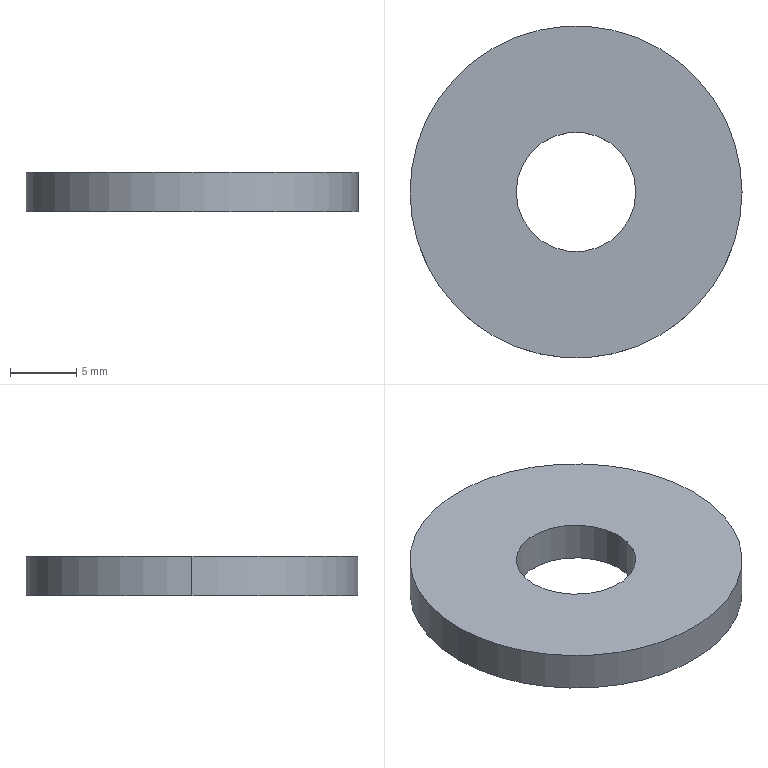Part | STEP file | Cuon T phu H01_15 | 1 solid | 6 faces | box 25 x 25 x 3 mm | volume 1282 mm3 | cylinder 4 | plane 2 | commonest cylinder face diameters 9 x2 25 x2
STEP:
#1=CARTESIAN_POINT('',(0.,0.,0.));
#2=DIRECTION('',(0.,0.,1.));
#3=DIRECTION('',(1.,0.,0.));
#4=AXIS2_PLACEMENT_3D('',#1,#2,#3);
#5=CARTESIAN_POINT('',(-4.5,0.,3.));
#6=VERTEX_POINT('',#5);
#7=CARTESIAN_POINT('',(-4.5,0.,0.));
#8=VERTEX_POINT('',#7);
#9=CARTESIAN_POINT('',(-4.5,0.,3.));
#10=DIRECTION('',(0.,0.,-1.));
#11=VECTOR('',#10,1.);
#12=LINE('',#9,#11);
#13=CARTESIAN_POINT('',(0.,0.,3.));
#14=DIRECTION('',(0.,0.,-1.));
#15=DIRECTION('',(-1.,0.,0.));
#16=AXIS2_PLACEMENT_3D('',#13,#14,#15);
#17=CYLINDRICAL_SURFACE('',#16,4.5);
#18=CARTESIAN_POINT('',(6.283,0.));
#19=DIRECTION('',(0.,1.));
#20=VECTOR('',#19,1.);
#21=LINE('',#18,#20);
#22=(GEOMETRIC_REPRESENTATION_CONTEXT(2)PARAMETRIC_REPRESENTATION_CONTEXT()REPRESENTATION_CONTEXT('',''));
#23=DEFINITIONAL_REPRESENTATION('',(#21),#22);
#24=PCURVE('',#17,#23);
#25=CARTESIAN_POINT('',(0.,0.,3.));
#26=DIRECTION('',(0.,0.,-1.));
#27=DIRECTION('',(-1.,0.,0.));
#28=AXIS2_PLACEMENT_3D('',#25,#26,#27);
#29=CYLINDRICAL_SURFACE('',#28,4.5);
#30=CARTESIAN_POINT('',(0.,0.));
#31=DIRECTION('',(0.,1.));
#32=VECTOR('',#31,1.);
#33=LINE('',#30,#32);
#34=(GEOMETRIC_REPRESENTATION_CONTEXT(2)PARAMETRIC_REPRESENTATION_CONTEXT()REPRESENTATION_CONTEXT('',''));
#35=DEFINITIONAL_REPRESENTATION('',(#33),#34);
#36=PCURVE('',#29,#35);
#37=SURFACE_CURVE('',#12,(#24,#36),.PCURVE_S1.);
#38=EDGE_CURVE('',#6,#8,#37,.T.);
#39=ORIENTED_EDGE('',*,*,#38,.T.);
#40=CARTESIAN_POINT('',(4.5,0.,0.));
#41=VERTEX_POINT('',#40);
#42=CARTESIAN_POINT('',(0.,0.,0.));
#43=DIRECTION('',(0.,0.,1.));
#44=DIRECTION('',(1.,0.,0.));
#45=AXIS2_PLACEMENT_3D('',#42,#43,#44);
#46=CIRCLE('',#45,4.5);
#47=CARTESIAN_POINT('',(9.425,3.));
#48=DIRECTION('',(-1.,0.));
#49=VECTOR('',#48,1.);
#50=LINE('',#47,#49);
#51=(GEOMETRIC_REPRESENTATION_CONTEXT(2)PARAMETRIC_REPRESENTATION_CONTEXT()REPRESENTATION_CONTEXT('',''));
#52=DEFINITIONAL_REPRESENTATION('',(#50),#51);
#53=PCURVE('',#17,#52);
#54=CARTESIAN_POINT('',(0.,0.,0.));
#55=DIRECTION('',(0.,0.,1.));
#56=DIRECTION('',(1.,0.,0.));
#57=AXIS2_PLACEMENT_3D('',#54,#55,#56);
#58=PLANE('',#57);
#59=CARTESIAN_POINT('',(0.,0.));
#60=DIRECTION('',(1.,0.));
#61=AXIS2_PLACEMENT_2D('',#59,#60);
#62=CIRCLE('',#61,4.5);
#63=(GEOMETRIC_REPRESENTATION_CONTEXT(2)PARAMETRIC_REPRESENTATION_CONTEXT()REPRESENTATION_CONTEXT('',''));
#64=DEFINITIONAL_REPRESENTATION('',(#62),#63);
#65=PCURVE('',#58,#64);
#66=SURFACE_CURVE('',#46,(#53,#65),.PCURVE_S1.);
#67=EDGE_CURVE('',#8,#41,#66,.T.);
#68=ORIENTED_EDGE('',*,*,#67,.T.);
#69=CARTESIAN_POINT('',(4.5,0.,3.));
#70=VERTEX_POINT('',#69);
#71=CARTESIAN_POINT('',(4.5,0.,3.));
#72=DIRECTION('',(0.,0.,-1.));
#73=VECTOR('',#72,1.);
#74=LINE('',#71,#73);
#75=CARTESIAN_POINT('',(3.142,0.));
#76=DIRECTION('',(0.,1.));
#77=VECTOR('',#76,1.);
#78=LINE('',#75,#77);
#79=(GEOMETRIC_REPRESENTATION_CONTEXT(2)PARAMETRIC_REPRESENTATION_CONTEXT()REPRESENTATION_CONTEXT('',''));
#80=DEFINITIONAL_REPRESENTATION('',(#78),#79);
#81=PCURVE('',#17,#80);
#82=CARTESIAN_POINT('',(3.142,0.));
#83=DIRECTION('',(0.,1.));
#84=VECTOR('',#83,1.);
#85=LINE('',#82,#84);
#86=(GEOMETRIC_REPRESENTATION_CONTEXT(2)PARAMETRIC_REPRESENTATION_CONTEXT()REPRESENTATION_CONTEXT('',''));
#87=DEFINITIONAL_REPRESENTATION('',(#85),#86);
#88=PCURVE('',#29,#87);
#89=SURFACE_CURVE('',#74,(#81,#88),.PCURVE_S1.);
#90=EDGE_CURVE('',#70,#41,#89,.T.);
#91=ORIENTED_EDGE('',*,*,#90,.F.);
#92=CARTESIAN_POINT('',(0.,0.,3.));
#93=DIRECTION('',(0.,0.,1.));
#94=DIRECTION('',(1.,0.,0.));
#95=AXIS2_PLACEMENT_3D('',#92,#93,#94);
#96=CIRCLE('',#95,4.5);
#97=CARTESIAN_POINT('',(9.425,0.));
#98=DIRECTION('',(-1.,0.));
#99=VECTOR('',#98,1.);
#100=LINE('',#97,#99);
#101=(GEOMETRIC_REPRESENTATION_CONTEXT(2)PARAMETRIC_REPRESENTATION_CONTEXT()REPRESENTATION_CONTEXT('',''));
#102=DEFINITIONAL_REPRESENTATION('',(#100),#101);
#103=PCURVE('',#17,#102);
#104=CARTESIAN_POINT('',(0.,0.,3.));
#105=DIRECTION('',(0.,0.,1.));
#106=DIRECTION('',(1.,0.,0.));
#107=AXIS2_PLACEMENT_3D('',#104,#105,#106);
#108=PLANE('',#107);
#109=CARTESIAN_POINT('',(0.,0.));
#110=DIRECTION('',(1.,0.));
#111=AXIS2_PLACEMENT_2D('',#109,#110);
#112=CIRCLE('',#111,4.5);
#113=(GEOMETRIC_REPRESENTATION_CONTEXT(2)PARAMETRIC_REPRESENTATION_CONTEXT()REPRESENTATION_CONTEXT('',''));
#114=DEFINITIONAL_REPRESENTATION('',(#112),#113);
#115=PCURVE('',#108,#114);
#116=SURFACE_CURVE('',#96,(#103,#115),.PCURVE_S1.);
#117=EDGE_CURVE('',#6,#70,#116,.T.);
#118=ORIENTED_EDGE('',*,*,#117,.F.);
#119=EDGE_LOOP('',(#39,#68,#91,#118));
#120=FACE_BOUND('',#119,.F.);
#121=ADVANCED_FACE('',(#120),#17,.F.);
#122=CARTESIAN_POINT('',(12.5,0.,3.));
#123=VERTEX_POINT('',#122);
#124=CARTESIAN_POINT('',(-12.5,0.,3.));
#125=VERTEX_POINT('',#124);
#126=CARTESIAN_POINT('',(0.,0.,3.));
#127=DIRECTION('',(0.,0.,1.));
#128=DIRECTION('',(1.,0.,0.));
#129=AXIS2_PLACEMENT_3D('',#126,#127,#128);
#130=CIRCLE('',#129,12.5);
#131=CARTESIAN_POINT('',(0.,0.,3.));
#132=DIRECTION('',(0.,0.,-1.));
#133=DIRECTION('',(-1.,0.,0.));
#134=AXIS2_PLACEMENT_3D('',#131,#132,#133);
#135=CYLINDRICAL_SURFACE('',#134,12.5);
#136=CARTESIAN_POINT('',(3.142,0.));
#137=DIRECTION('',(-1.,0.));
#138=VECTOR('',#137,1.);
#139=LINE('',#136,#138);
#140=(GEOMETRIC_REPRESENTATION_CONTEXT(2)PARAMETRIC_REPRESENTATION_CONTEXT()REPRESENTATION_CONTEXT('',''));
#141=DEFINITIONAL_REPRESENTATION('',(#139),#140);
#142=PCURVE('',#135,#141);
#143=CARTESIAN_POINT('',(0.,0.));
#144=DIRECTION('',(1.,0.));
#145=AXIS2_PLACEMENT_2D('',#143,#144);
#146=CIRCLE('',#145,12.5);
#147=(GEOMETRIC_REPRESENTATION_CONTEXT(2)PARAMETRIC_REPRESENTATION_CONTEXT()REPRESENTATION_CONTEXT('',''));
#148=DEFINITIONAL_REPRESENTATION('',(#146),#147);
#149=PCURVE('',#108,#148);
#150=SURFACE_CURVE('',#130,(#142,#149),.PCURVE_S1.);
#151=EDGE_CURVE('',#123,#125,#150,.T.);
#152=ORIENTED_EDGE('',*,*,#151,.F.);
#153=CARTESIAN_POINT('',(12.5,0.,0.));
#154=VERTEX_POINT('',#153);
#155=CARTESIAN_POINT('',(12.5,0.,3.));
#156=DIRECTION('',(0.,0.,-1.));
#157=VECTOR('',#156,1.);
#158=LINE('',#155,#157);
#159=CARTESIAN_POINT('',(3.142,0.));
#160=DIRECTION('',(0.,1.));
#161=VECTOR('',#160,1.);
#162=LINE('',#159,#161);
#163=(GEOMETRIC_REPRESENTATION_CONTEXT(2)PARAMETRIC_REPRESENTATION_CONTEXT()REPRESENTATION_CONTEXT('',''));
#164=DEFINITIONAL_REPRESENTATION('',(#162),#163);
#165=PCURVE('',#135,#164);
#166=CARTESIAN_POINT('',(0.,0.,3.));
#167=DIRECTION('',(0.,0.,-1.));
#168=DIRECTION('',(-1.,0.,0.));
#169=AXIS2_PLACEMENT_3D('',#166,#167,#168);
#170=CYLINDRICAL_SURFACE('',#169,12.5);
#171=CARTESIAN_POINT('',(3.142,0.));
#172=DIRECTION('',(0.,1.));
#173=VECTOR('',#172,1.);
#174=LINE('',#171,#173);
#175=(GEOMETRIC_REPRESENTATION_CONTEXT(2)PARAMETRIC_REPRESENTATION_CONTEXT()REPRESENTATION_CONTEXT('',''));
#176=DEFINITIONAL_REPRESENTATION('',(#174),#175);
#177=PCURVE('',#170,#176);
#178=SURFACE_CURVE('',#158,(#165,#177),.PCURVE_S1.);
#179=EDGE_CURVE('',#123,#154,#178,.T.);
#180=ORIENTED_EDGE('',*,*,#179,.T.);
#181=CARTESIAN_POINT('',(-12.5,0.,0.));
#182=VERTEX_POINT('',#181);
#183=CARTESIAN_POINT('',(0.,0.,0.));
#184=DIRECTION('',(0.,0.,1.));
#185=DIRECTION('',(1.,0.,0.));
#186=AXIS2_PLACEMENT_3D('',#183,#184,#185);
#187=CIRCLE('',#186,12.5);
#188=CARTESIAN_POINT('',(3.142,3.));
#189=DIRECTION('',(-1.,0.));
#190=VECTOR('',#189,1.);
#191=LINE('',#188,#190);
#192=(GEOMETRIC_REPRESENTATION_CONTEXT(2)PARAMETRIC_REPRESENTATION_CONTEXT()REPRESENTATION_CONTEXT('',''));
#193=DEFINITIONAL_REPRESENTATION('',(#191),#192);
#194=PCURVE('',#135,#193);
#195=CARTESIAN_POINT('',(0.,0.));
#196=DIRECTION('',(1.,0.));
#197=AXIS2_PLACEMENT_2D('',#195,#196);
#198=CIRCLE('',#197,12.5);
#199=(GEOMETRIC_REPRESENTATION_CONTEXT(2)PARAMETRIC_REPRESENTATION_CONTEXT()REPRESENTATION_CONTEXT('',''));
#200=DEFINITIONAL_REPRESENTATION('',(#198),#199);
#201=PCURVE('',#58,#200);
#202=SURFACE_CURVE('',#187,(#194,#201),.PCURVE_S1.);
#203=EDGE_CURVE('',#154,#182,#202,.T.);
#204=ORIENTED_EDGE('',*,*,#203,.T.);
#205=CARTESIAN_POINT('',(-12.5,0.,3.));
#206=DIRECTION('',(0.,0.,-1.));
#207=VECTOR('',#206,1.);
#208=LINE('',#205,#207);
#209=CARTESIAN_POINT('',(0.,0.));
#210=DIRECTION('',(0.,1.));
#211=VECTOR('',#210,1.);
#212=LINE('',#209,#211);
#213=(GEOMETRIC_REPRESENTATION_CONTEXT(2)PARAMETRIC_REPRESENTATION_CONTEXT()REPRESENTATION_CONTEXT('',''));
#214=DEFINITIONAL_REPRESENTATION('',(#212),#213);
#215=PCURVE('',#135,#214);
#216=CARTESIAN_POINT('',(6.283,0.));
#217=DIRECTION('',(0.,1.));
#218=VECTOR('',#217,1.);
#219=LINE('',#216,#218);
#220=(GEOMETRIC_REPRESENTATION_CONTEXT(2)PARAMETRIC_REPRESENTATION_CONTEXT()REPRESENTATION_CONTEXT('',''));
#221=DEFINITIONAL_REPRESENTATION('',(#219),#220);
#222=PCURVE('',#170,#221);
#223=SURFACE_CURVE('',#208,(#215,#222),.PCURVE_S1.);
#224=EDGE_CURVE('',#125,#182,#223,.T.);
#225=ORIENTED_EDGE('',*,*,#224,.F.);
#226=EDGE_LOOP('',(#152,#180,#204,#225));
#227=FACE_BOUND('',#226,.T.);
#228=ADVANCED_FACE('',(#227),#135,.T.);
#229=CARTESIAN_POINT('',(0.,0.,3.));
#230=DIRECTION('',(0.,0.,1.));
#231=DIRECTION('',(1.,0.,0.));
#232=AXIS2_PLACEMENT_3D('',#229,#230,#231);
#233=CIRCLE('',#232,12.5);
#234=CARTESIAN_POINT('',(0.,0.));
#235=DIRECTION('',(1.,0.));
#236=AXIS2_PLACEMENT_2D('',#234,#235);
#237=CIRCLE('',#236,12.5);
#238=(GEOMETRIC_REPRESENTATION_CONTEXT(2)PARAMETRIC_REPRESENTATION_CONTEXT()REPRESENTATION_CONTEXT('',''));
#239=DEFINITIONAL_REPRESENTATION('',(#237),#238);
#240=PCURVE('',#108,#239);
#241=CARTESIAN_POINT('',(9.425,0.));
#242=DIRECTION('',(-1.,0.));
#243=VECTOR('',#242,1.);
#244=LINE('',#241,#243);
#245=(GEOMETRIC_REPRESENTATION_CONTEXT(2)PARAMETRIC_REPRESENTATION_CONTEXT()REPRESENTATION_CONTEXT('',''));
#246=DEFINITIONAL_REPRESENTATION('',(#244),#245);
#247=PCURVE('',#170,#246);
#248=SURFACE_CURVE('',#233,(#240,#247),.PCURVE_S1.);
#249=EDGE_CURVE('',#125,#123,#248,.T.);
#250=ORIENTED_EDGE('',*,*,#249,.T.);
#251=ORIENTED_EDGE('',*,*,#151,.T.);
#252=EDGE_LOOP('',(#250,#251));
#253=FACE_BOUND('',#252,.T.);
#254=ORIENTED_EDGE('',*,*,#117,.F.);
#255=CARTESIAN_POINT('',(0.,0.,3.));
#256=DIRECTION('',(0.,0.,1.));
#257=DIRECTION('',(1.,0.,0.));
#258=AXIS2_PLACEMENT_3D('',#255,#256,#257);
#259=CIRCLE('',#258,4.5);
#260=CARTESIAN_POINT('',(0.,0.));
#261=DIRECTION('',(1.,0.));
#262=AXIS2_PLACEMENT_2D('',#260,#261);
#263=CIRCLE('',#262,4.5);
#264=(GEOMETRIC_REPRESENTATION_CONTEXT(2)PARAMETRIC_REPRESENTATION_CONTEXT()REPRESENTATION_CONTEXT('',''));
#265=DEFINITIONAL_REPRESENTATION('',(#263),#264);
#266=PCURVE('',#108,#265);
#267=CARTESIAN_POINT('',(3.142,0.));
#268=DIRECTION('',(-1.,0.));
#269=VECTOR('',#268,1.);
#270=LINE('',#267,#269);
#271=(GEOMETRIC_REPRESENTATION_CONTEXT(2)PARAMETRIC_REPRESENTATION_CONTEXT()REPRESENTATION_CONTEXT('',''));
#272=DEFINITIONAL_REPRESENTATION('',(#270),#271);
#273=PCURVE('',#29,#272);
#274=SURFACE_CURVE('',#259,(#266,#273),.PCURVE_S1.);
#275=EDGE_CURVE('',#70,#6,#274,.T.);
#276=ORIENTED_EDGE('',*,*,#275,.F.);
#277=EDGE_LOOP('',(#254,#276));
#278=FACE_BOUND('',#277,.T.);
#279=ADVANCED_FACE('',(#253,#278),#108,.T.);
#280=CARTESIAN_POINT('',(0.,0.,0.));
#281=DIRECTION('',(0.,0.,1.));
#282=DIRECTION('',(1.,0.,0.));
#283=AXIS2_PLACEMENT_3D('',#280,#281,#282);
#284=CIRCLE('',#283,12.5);
#285=CARTESIAN_POINT('',(0.,0.));
#286=DIRECTION('',(1.,0.));
#287=AXIS2_PLACEMENT_2D('',#285,#286);
#288=CIRCLE('',#287,12.5);
#289=(GEOMETRIC_REPRESENTATION_CONTEXT(2)PARAMETRIC_REPRESENTATION_CONTEXT()REPRESENTATION_CONTEXT('',''));
#290=DEFINITIONAL_REPRESENTATION('',(#288),#289);
#291=PCURVE('',#58,#290);
#292=CARTESIAN_POINT('',(9.425,3.));
#293=DIRECTION('',(-1.,0.));
#294=VECTOR('',#293,1.);
#295=LINE('',#292,#294);
#296=(GEOMETRIC_REPRESENTATION_CONTEXT(2)PARAMETRIC_REPRESENTATION_CONTEXT()REPRESENTATION_CONTEXT('',''));
#297=DEFINITIONAL_REPRESENTATION('',(#295),#296);
#298=PCURVE('',#170,#297);
#299=SURFACE_CURVE('',#284,(#291,#298),.PCURVE_S1.);
#300=EDGE_CURVE('',#182,#154,#299,.T.);
#301=ORIENTED_EDGE('',*,*,#300,.F.);
#302=ORIENTED_EDGE('',*,*,#203,.F.);
#303=EDGE_LOOP('',(#301,#302));
#304=FACE_BOUND('',#303,.T.);
#305=ORIENTED_EDGE('',*,*,#67,.T.);
#306=CARTESIAN_POINT('',(0.,0.,0.));
#307=DIRECTION('',(0.,0.,1.));
#308=DIRECTION('',(1.,0.,0.));
#309=AXIS2_PLACEMENT_3D('',#306,#307,#308);
#310=CIRCLE('',#309,4.5);
#311=CARTESIAN_POINT('',(0.,0.));
#312=DIRECTION('',(1.,0.));
#313=AXIS2_PLACEMENT_2D('',#311,#312);
#314=CIRCLE('',#313,4.5);
#315=(GEOMETRIC_REPRESENTATION_CONTEXT(2)PARAMETRIC_REPRESENTATION_CONTEXT()REPRESENTATION_CONTEXT('',''));
#316=DEFINITIONAL_REPRESENTATION('',(#314),#315);
#317=PCURVE('',#58,#316);
#318=CARTESIAN_POINT('',(3.142,3.));
#319=DIRECTION('',(-1.,0.));
#320=VECTOR('',#319,1.);
#321=LINE('',#318,#320);
#322=(GEOMETRIC_REPRESENTATION_CONTEXT(2)PARAMETRIC_REPRESENTATION_CONTEXT()REPRESENTATION_CONTEXT('',''));
#323=DEFINITIONAL_REPRESENTATION('',(#321),#322);
#324=PCURVE('',#29,#323);
#325=SURFACE_CURVE('',#310,(#317,#324),.PCURVE_S1.);
#326=EDGE_CURVE('',#41,#8,#325,.T.);
#327=ORIENTED_EDGE('',*,*,#326,.T.);
#328=EDGE_LOOP('',(#305,#327));
#329=FACE_BOUND('',#328,.T.);
#330=ADVANCED_FACE('',(#304,#329),#58,.F.);
#331=ORIENTED_EDGE('',*,*,#179,.F.);
#332=ORIENTED_EDGE('',*,*,#249,.F.);
#333=ORIENTED_EDGE('',*,*,#224,.T.);
#334=ORIENTED_EDGE('',*,*,#300,.T.);
#335=EDGE_LOOP('',(#331,#332,#333,#334));
#336=FACE_BOUND('',#335,.T.);
#337=ADVANCED_FACE('',(#336),#170,.T.);
#338=ORIENTED_EDGE('',*,*,#326,.T.);
#339=ORIENTED_EDGE('',*,*,#38,.F.);
#340=ORIENTED_EDGE('',*,*,#275,.F.);
#341=ORIENTED_EDGE('',*,*,#90,.T.);
#342=EDGE_LOOP('',(#338,#339,#340,#341));
#343=FACE_BOUND('',#342,.F.);
#344=ADVANCED_FACE('',(#343),#29,.F.);
#345=CLOSED_SHELL('',(#121,#228,#279,#330,#337,#344));
#346=MANIFOLD_SOLID_BREP('',#345);
#347=(LENGTH_UNIT()NAMED_UNIT(*)SI_UNIT(.MILLI.,.METRE.));
#348=UNCERTAINTY_MEASURE_WITH_UNIT(LENGTH_MEASURE(0.0000001),#347,'','');
#349=(NAMED_UNIT(*)PLANE_ANGLE_UNIT()SI_UNIT($,.RADIAN.));
#350=(NAMED_UNIT(*)SI_UNIT($,.STERADIAN.)SOLID_ANGLE_UNIT());
#351=(GEOMETRIC_REPRESENTATION_CONTEXT(3)GLOBAL_UNCERTAINTY_ASSIGNED_CONTEXT((#348))GLOBAL_UNIT_ASSIGNED_CONTEXT((#347,#349,#350))REPRESENTATION_CONTEXT('',''));
#352=ADVANCED_BREP_SHAPE_REPRESENTATION('',(#4,#346),#351);